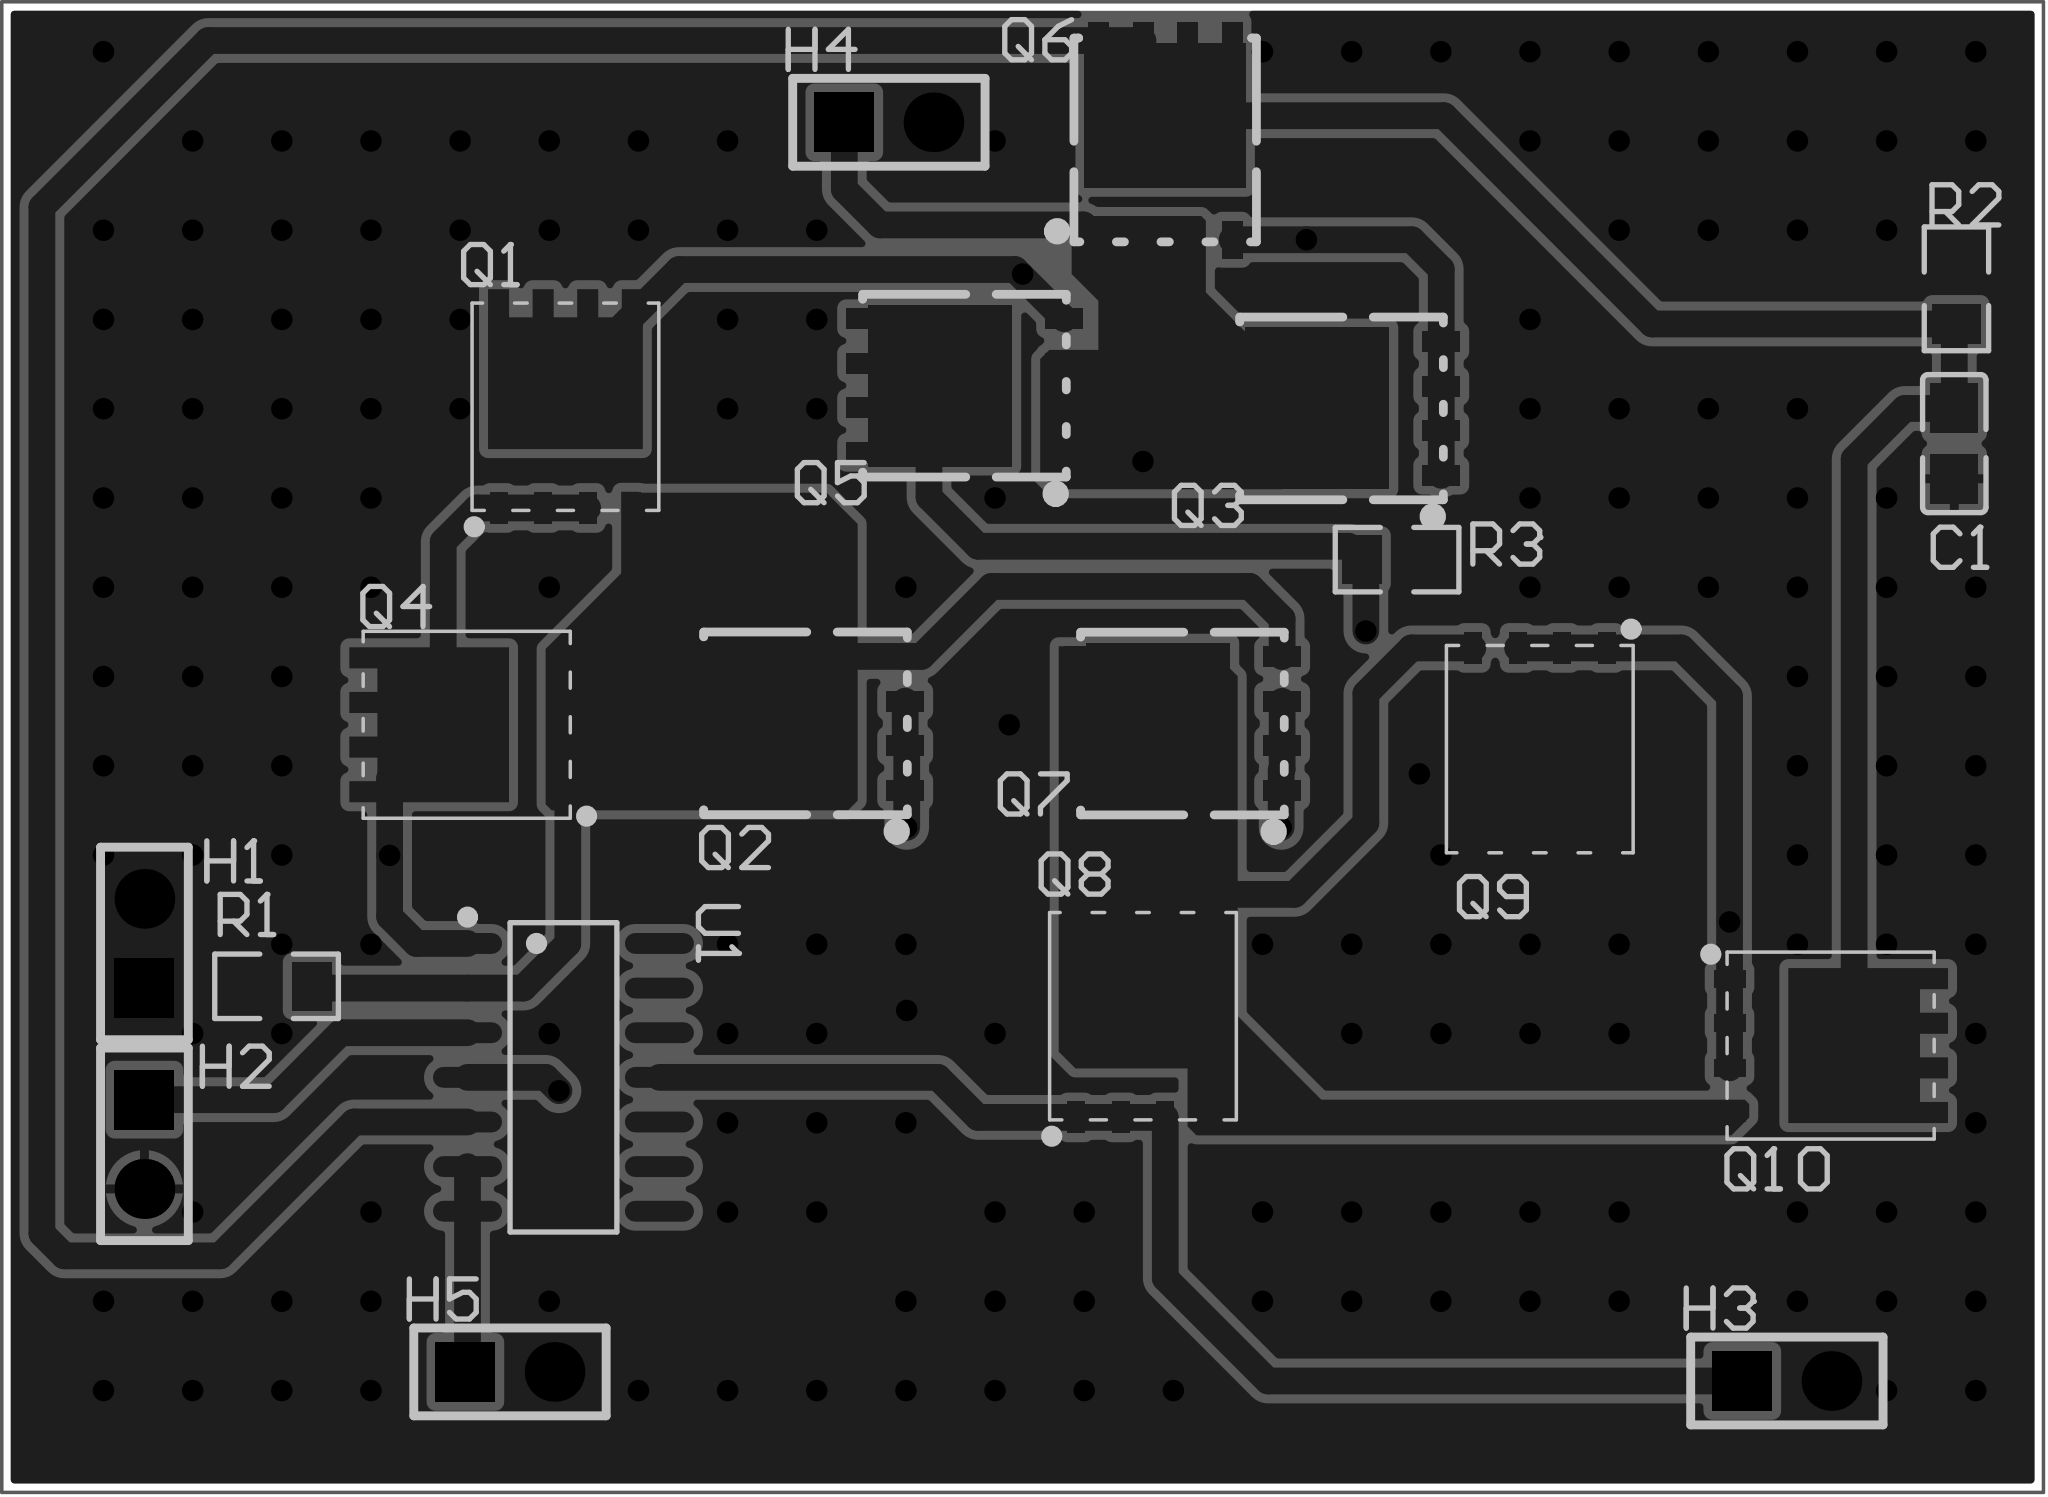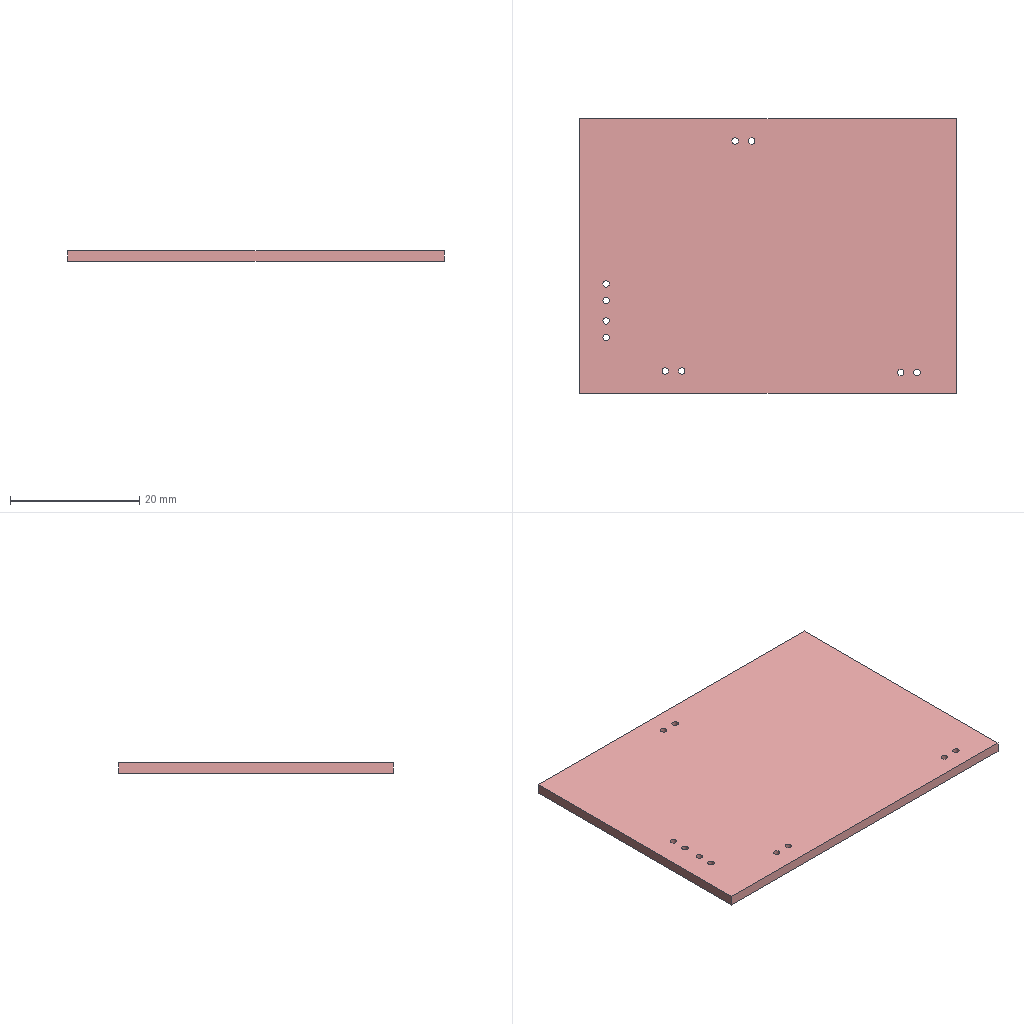Circuit board layout | Altium Designer | box 58.2 x 42.4 x 1.6 mm
Layer stack:
# Altium Designer layer stack of  (unit mm; dielectric type: 0 none, 1 core, 2 prepreg, 3 surface material)
index,name,kind,layer,copper_thickness_mm,dielectric_type,dielectric_thickness_mm,dielectric_material,dielectric_constant
0,Top Paste Mask Layer,other,,,,,,
1,Top Silkscreen Layer,other,,,,,,
2,Top Solder Mask Layer,dielectric,,,3,0.01,,3.3
3,Top Layer,copper,Top Layer,0.035,,,,
4,Dielectric1,dielectric,,,3,1.51,FR4,4.5
5,Bottom Layer,copper,Bottom Layer,0.035,,,,
6,Bottom Solder Mask Layer,dielectric,,,3,0.01,,3.3
7,Bottom Silkscreen Layer,other,,,,,,
8,Bottom Paste Mask Layer,other,,,,,,
# drill layer pairs: low layer,high layer
drill_pair,Top Layer,Bottom Layer
Part placement:
Designator,Comment,Layer,Footprint,Center-X(mm),Center-Y(mm),Rotation
C1,3.3nF,TopLayer,C0805,135.128,108.839,90
H1,,TopLayer,HDR-TH_2P-P2.54-V-F,83.566,94.615,90
H2,,TopLayer,HDR-TH_2P-P2.54-V-F,83.566,88.9,270
H3,,TopLayer,HDR-TH_2P-P2.54-V-F,130.358,82.165,0
H4,,TopLayer,HDR-TH_2P-P2.54-V-F,104.775,117.983,0
H5,,TopLayer,HDR-TH_2P-P2.54-V-F,93.98,82.423,0
Q1,SI7336ADP-T1-E3-MS,TopLayer,TDSON-8_L5.9-W5.2-P1.27-BL-1,95.56,108.901,0
Q2,AON6407,TopLayer,PDFN-8_L4.9-W5.8-P1.27-LS6.1-BL,102.405,100.881,90
Q3,AON6407,TopLayer,PDFN-8_L4.9-W5.8-P1.27-LS6.1-BL,117.677,109.843,90
Q4,SI7336ADP-T1-E3-MS,TopLayer,TDSON-8_L5.9-W5.2-P1.27-BL-1,93.735,100.838,90
Q5,AON6407,TopLayer,PDFN-8_L4.9-W5.8-P1.27-LS6.1-BL,106.934,110.49,90
Q6,AON6407,TopLayer,PDFN-8_L4.9-W5.8-P1.27-LS6.1-BL,112.649,117.475,0
Q7,AON6407,TopLayer,PDFN-8_L4.9-W5.8-P1.27-LS6.1-BL,113.144,100.875,90
Q8,SI7336ADP-T1-E3-MS,TopLayer,TDSON-8_L5.9-W5.2-P1.27-BL-1,112.014,91.558,0
Q9,SI7336ADP-T1-E3-MS,TopLayer,TDSON-8_L5.9-W5.2-P1.27-BL-1,123.319,101.132,180
Q10,SI7336ADP-T1-E3-MS,TopLayer,TDSON-8_L5.9-W5.2-P1.27-BL-1,130.618,91.709,270
R1,47K,TopLayer,R0805,87.33,93.396,0
R2,1e9,TopLayer,R0805,135.189,113.244,270
R3,1e6,TopLayer,R0805,119.253,105.537,180
U1,TL084,TopLayer,SOP-14_L8.6-W3.9-P1.27-LS6.0-BL,95.504,90.805,270
Pad and via stacks:
# Altium Designer via and pad stacks of  (unit mm). Each distinct definition once, with the count of objects using it.
# via: kind,start_layer,end_layer,hole_mm,diameter_mm,mode(0 simple;1 top-mid-bottom;2 full stack),diameter_per_layer,count,example_net
# pad: kind,layer,hole_mm,hole_type(0 round;1 square;2 slot),plating,top_size,top_shape(1 round;2 rect;3 octagon;9 rounded rect),mid_size,bottom_size,mode,footprint,size_per_layer,count,example
pad,Top Layer,0,0,plated,1.41x1.35,2,1.41x1.35,1.41x1.35,0,C0805,,2,C1.2
pad,Top Layer,0,0,plated,1.638x1.638,1,1.638x1.638,1.638x1.638,0,TDSON-8_L5.9-W5.2-P1.27-BL-1,,5,Q1.5
pad,Top Layer,0,0,plated,0.5x0.9,2,0.5x0.9,0.5x0.9,0,TDSON-8_L5.9-W5.2-P1.27-BL-1,,20,Q1.4
pad,Top Layer,0,0,plated,4.6x4.1,2,4.6x4.1,4.6x4.1,0,PDFN-8_L4.9-W5.8-P1.27-LS6.1-BL,,5,Q2.9
pad,Top Layer,0,0,plated,0.58x1.08,2,0.58x1.08,0.58x1.08,0,PDFN-8_L4.9-W5.8-P1.27-LS6.1-BL,,20,Q2.5
pad,Top Layer,0,0,plated,0.58x1.079,2,0.58x1.079,0.58x1.079,0,PDFN-8_L4.9-W5.8-P1.27-LS6.1-BL,,20,Q2.1
pad,Top Layer,0,0,plated,1.133x1.377,2,1.133x1.377,1.133x1.377,0,R0805,,6,R1.2
pad,Top Layer,0,0,plated,0.595x1.968,1,0.595x1.968,0.595x1.968,0,SOP-14_L8.6-W3.9-P1.27-LS6.0-BL,,14,U1.1
pad,Multi-Layer,1,0,plated,1.7x1.7,2,1.7x1.7,1.7x1.7,0,HDR-TH_2P-P2.54-V-F,,5,H1.1
pad,Multi-Layer,1,0,plated,1.7x1.7,1,1.7x1.7,1.7x1.7,0,HDR-TH_2P-P2.54-V-F,,5,H1.2
via,Top Layer,Bottom Layer,0.3048,0.61,0,,180,$1N8
Copper pours:
name,layer,net,type(0 solid;1 hatched;2 none)
Top Layer-GND,Top Layer,GND,0
Bottom Layer-GND,Bottom Layer,GND,0